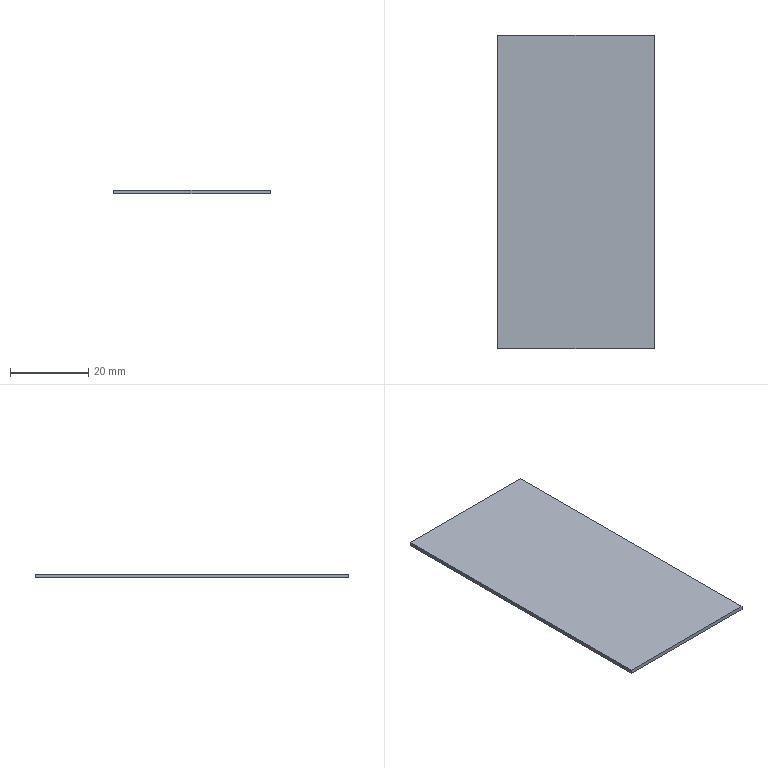Part | SolidWorks | features Extrusion 1 | 1 solid | 6 faces | box 40 x 80 x 1 mm | volume 3200 mm3 | plane 6
STEP:
#1=CARTESIAN_POINT('',(20.,-40.,-0.5));
#2=VERTEX_POINT('',#1);
#3=CARTESIAN_POINT('',(20.,40.,-0.5));
#4=VERTEX_POINT('',#3);
#5=CARTESIAN_POINT('',(20.,-40.,-0.5));
#6=DIRECTION('',(0.,1.,0.));
#7=VECTOR('',#6,1000.);
#8=LINE('',#5,#7);
#9=EDGE_CURVE('',#2,#4,#8,.T.);
#10=ORIENTED_EDGE('',*,*,#9,.T.);
#11=CARTESIAN_POINT('',(20.,40.,0.5));
#12=VERTEX_POINT('',#11);
#13=CARTESIAN_POINT('',(20.,40.,0.5));
#14=DIRECTION('',(0.,0.,-1.));
#15=VECTOR('',#14,1000.);
#16=LINE('',#13,#15);
#17=EDGE_CURVE('',#12,#4,#16,.T.);
#18=ORIENTED_EDGE('',*,*,#17,.F.);
#19=CARTESIAN_POINT('',(20.,-40.,0.5));
#20=VERTEX_POINT('',#19);
#21=CARTESIAN_POINT('',(20.,-40.,0.5));
#22=DIRECTION('',(0.,1.,0.));
#23=VECTOR('',#22,1000.);
#24=LINE('',#21,#23);
#25=EDGE_CURVE('',#20,#12,#24,.T.);
#26=ORIENTED_EDGE('',*,*,#25,.F.);
#27=CARTESIAN_POINT('',(20.,-40.,0.5));
#28=DIRECTION('',(0.,0.,-1.));
#29=VECTOR('',#28,1000.);
#30=LINE('',#27,#29);
#31=EDGE_CURVE('',#20,#2,#30,.T.);
#32=ORIENTED_EDGE('',*,*,#31,.T.);
#33=EDGE_LOOP('',(#10,#18,#26,#32));
#34=FACE_OUTER_BOUND('',#33,.T.);
#35=CARTESIAN_POINT('',(20.,-40.,0.5));
#36=DIRECTION('',(-1.,0.,0.));
#37=DIRECTION('',(0.,0.,1.));
#38=AXIS2_PLACEMENT_3D('',#35,#36,#37);
#39=PLANE('',#38);
#40=ADVANCED_FACE('',(#34),#39,.F.);
#41=CARTESIAN_POINT('',(-20.,40.,-0.5));
#42=VERTEX_POINT('',#41);
#43=CARTESIAN_POINT('',(-20.,40.,-0.5));
#44=DIRECTION('',(-1.,0.,0.));
#45=VECTOR('',#44,1000.);
#46=LINE('',#43,#45);
#47=EDGE_CURVE('',#4,#42,#46,.T.);
#48=ORIENTED_EDGE('',*,*,#47,.T.);
#49=CARTESIAN_POINT('',(-20.,40.,0.5));
#50=VERTEX_POINT('',#49);
#51=CARTESIAN_POINT('',(-20.,40.,0.5));
#52=DIRECTION('',(0.,0.,-1.));
#53=VECTOR('',#52,1000.);
#54=LINE('',#51,#53);
#55=EDGE_CURVE('',#50,#42,#54,.T.);
#56=ORIENTED_EDGE('',*,*,#55,.F.);
#57=CARTESIAN_POINT('',(-20.,40.,0.5));
#58=DIRECTION('',(-1.,0.,0.));
#59=VECTOR('',#58,1000.);
#60=LINE('',#57,#59);
#61=EDGE_CURVE('',#12,#50,#60,.T.);
#62=ORIENTED_EDGE('',*,*,#61,.F.);
#63=ORIENTED_EDGE('',*,*,#17,.T.);
#64=EDGE_LOOP('',(#48,#56,#62,#63));
#65=FACE_OUTER_BOUND('',#64,.T.);
#66=CARTESIAN_POINT('',(-20.,40.,0.5));
#67=DIRECTION('',(0.,-1.,0.));
#68=DIRECTION('',(0.,0.,-1.));
#69=AXIS2_PLACEMENT_3D('',#66,#67,#68);
#70=PLANE('',#69);
#71=ADVANCED_FACE('',(#65),#70,.F.);
#72=CARTESIAN_POINT('',(-20.,-40.,-0.5));
#73=VERTEX_POINT('',#72);
#74=CARTESIAN_POINT('',(-20.,-40.,-0.5));
#75=DIRECTION('',(0.,-1.,0.));
#76=VECTOR('',#75,1000.);
#77=LINE('',#74,#76);
#78=EDGE_CURVE('',#42,#73,#77,.T.);
#79=ORIENTED_EDGE('',*,*,#78,.T.);
#80=CARTESIAN_POINT('',(-20.,-40.,0.5));
#81=VERTEX_POINT('',#80);
#82=CARTESIAN_POINT('',(-20.,-40.,0.5));
#83=DIRECTION('',(0.,0.,-1.));
#84=VECTOR('',#83,1000.);
#85=LINE('',#82,#84);
#86=EDGE_CURVE('',#81,#73,#85,.T.);
#87=ORIENTED_EDGE('',*,*,#86,.F.);
#88=CARTESIAN_POINT('',(-20.,-40.,0.5));
#89=DIRECTION('',(0.,-1.,0.));
#90=VECTOR('',#89,1000.);
#91=LINE('',#88,#90);
#92=EDGE_CURVE('',#50,#81,#91,.T.);
#93=ORIENTED_EDGE('',*,*,#92,.F.);
#94=ORIENTED_EDGE('',*,*,#55,.T.);
#95=EDGE_LOOP('',(#79,#87,#93,#94));
#96=FACE_OUTER_BOUND('',#95,.T.);
#97=CARTESIAN_POINT('',(-20.,-40.,0.5));
#98=DIRECTION('',(1.,0.,0.));
#99=DIRECTION('',(0.,0.,-1.));
#100=AXIS2_PLACEMENT_3D('',#97,#98,#99);
#101=PLANE('',#100);
#102=ADVANCED_FACE('',(#96),#101,.F.);
#103=CARTESIAN_POINT('',(-20.,-40.,-0.5));
#104=DIRECTION('',(1.,0.,0.));
#105=VECTOR('',#104,1000.);
#106=LINE('',#103,#105);
#107=EDGE_CURVE('',#73,#2,#106,.T.);
#108=ORIENTED_EDGE('',*,*,#107,.T.);
#109=ORIENTED_EDGE('',*,*,#31,.F.);
#110=CARTESIAN_POINT('',(-20.,-40.,0.5));
#111=DIRECTION('',(1.,0.,0.));
#112=VECTOR('',#111,1000.);
#113=LINE('',#110,#112);
#114=EDGE_CURVE('',#81,#20,#113,.T.);
#115=ORIENTED_EDGE('',*,*,#114,.F.);
#116=ORIENTED_EDGE('',*,*,#86,.T.);
#117=EDGE_LOOP('',(#108,#109,#115,#116));
#118=FACE_OUTER_BOUND('',#117,.T.);
#119=CARTESIAN_POINT('',(-20.,-40.,0.5));
#120=DIRECTION('',(0.,1.,0.));
#121=DIRECTION('',(0.,0.,1.));
#122=AXIS2_PLACEMENT_3D('',#119,#120,#121);
#123=PLANE('',#122);
#124=ADVANCED_FACE('',(#118),#123,.F.);
#125=ORIENTED_EDGE('',*,*,#25,.T.);
#126=ORIENTED_EDGE('',*,*,#61,.T.);
#127=ORIENTED_EDGE('',*,*,#92,.T.);
#128=ORIENTED_EDGE('',*,*,#114,.T.);
#129=EDGE_LOOP('',(#125,#126,#127,#128));
#130=FACE_OUTER_BOUND('',#129,.T.);
#131=CARTESIAN_POINT('',(0.,0.,0.5));
#132=DIRECTION('',(0.,0.,-1.));
#133=DIRECTION('',(-1.,0.,0.));
#134=AXIS2_PLACEMENT_3D('',#131,#132,#133);
#135=PLANE('',#134);
#136=ADVANCED_FACE('',(#130),#135,.F.);
#137=ORIENTED_EDGE('',*,*,#9,.F.);
#138=ORIENTED_EDGE('',*,*,#107,.F.);
#139=ORIENTED_EDGE('',*,*,#78,.F.);
#140=ORIENTED_EDGE('',*,*,#47,.F.);
#141=EDGE_LOOP('',(#137,#138,#139,#140));
#142=FACE_OUTER_BOUND('',#141,.T.);
#143=CARTESIAN_POINT('',(0.,0.,-0.5));
#144=DIRECTION('',(0.,0.,-1.));
#145=DIRECTION('',(-1.,0.,0.));
#146=AXIS2_PLACEMENT_3D('',#143,#144,#145);
#147=PLANE('',#146);
#148=ADVANCED_FACE('',(#142),#147,.T.);
#149=CLOSED_SHELL('',(#40,#71,#102,#124,#136,#148));
#150=MANIFOLD_SOLID_BREP('',#149);
#151=CARTESIAN_POINT('',(0.,0.,0.));
#152=DIRECTION('',(0.,0.,1.));
#153=DIRECTION('',(1.,0.,0.));
#154=AXIS2_PLACEMENT_3D('',#151,#152,#153);
#155=(LENGTH_UNIT()NAMED_UNIT(*)SI_UNIT(.MILLI.,.METRE.));
#156=UNCERTAINTY_MEASURE_WITH_UNIT(LENGTH_MEASURE(0.00001),#155,'','');
#157=(NAMED_UNIT(*)PLANE_ANGLE_UNIT()SI_UNIT($,.RADIAN.));
#158=(NAMED_UNIT(*)SI_UNIT($,.STERADIAN.)SOLID_ANGLE_UNIT());
#159=(GEOMETRIC_REPRESENTATION_CONTEXT(3)GLOBAL_UNCERTAINTY_ASSIGNED_CONTEXT((#156))GLOBAL_UNIT_ASSIGNED_CONTEXT((#155,#157,#158))REPRESENTATION_CONTEXT('',''));
#160=ADVANCED_BREP_SHAPE_REPRESENTATION('',(#150,#154),#159);